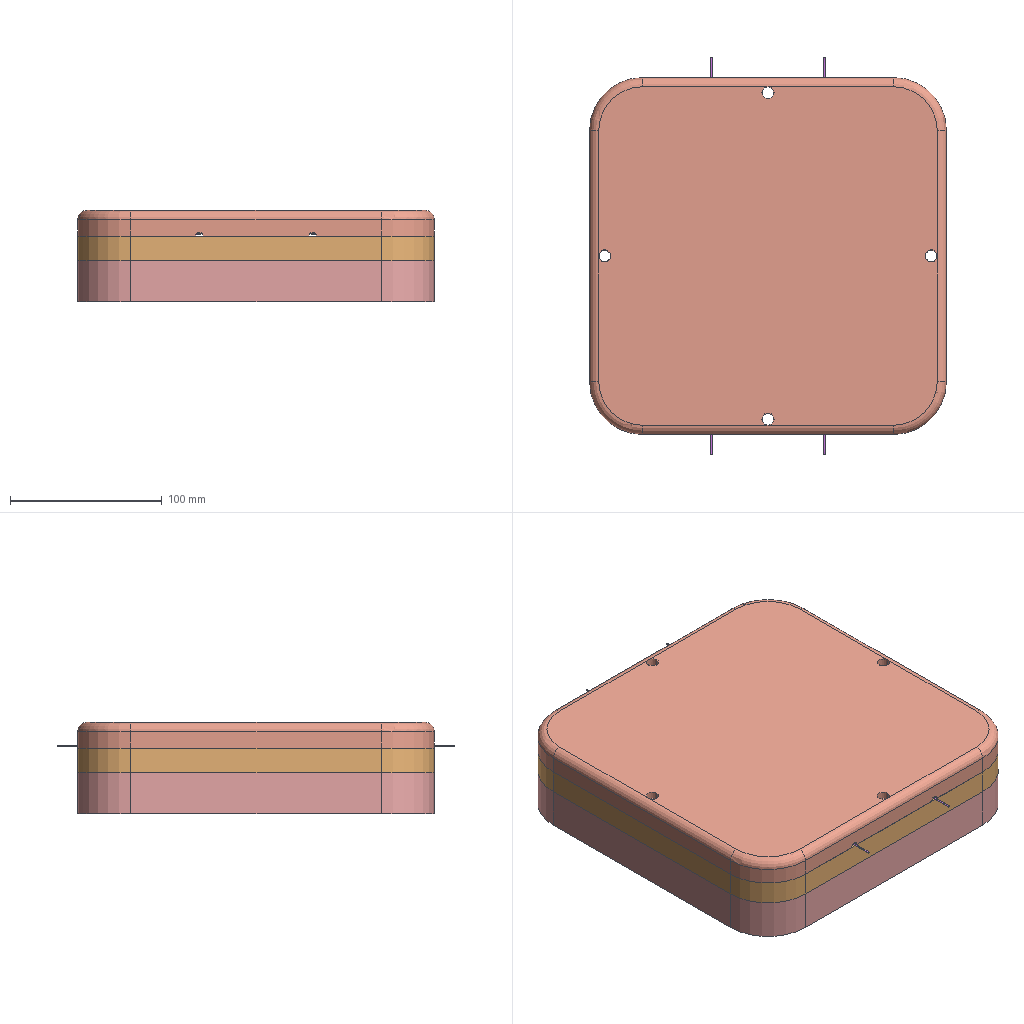Assembly | SolidWorks | 15 different items | 131 placed | box 235 x 262 x 60 mm
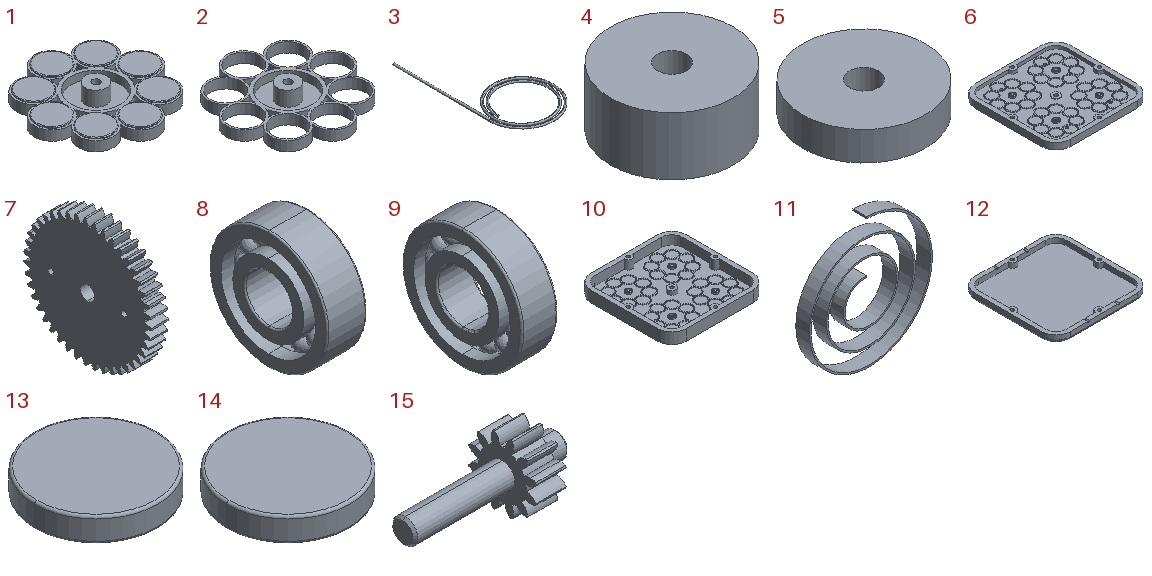Parts list (item | name | quantity | parent item | size | volume | features):
1 | (subassembly) | x4 | - | 100 x 100 x 14 mm | 35245 mm3 | features ReferencePattern 6, LocalCirPattern 1
2 | - | x4 | in 1 | 100 x 100 x 14 mm | 15045 mm3 | features ICE 2, Extrusion 1
3 | - | x4 | - | 33.004 x 66.506 x 1 mm | 182.398 mm3 | features Helix 1, ICE 1, Sweep 1
4 | - | x32 | - | 25.4 x 25.4 x 12 mm | 5741 mm3 | features Extrusion 1
5 | - | x32 | - | 25.4 x 25.4 x 6 mm | 2871 mm3 | features Extrusion 1
6 | - | x1 | - | 235 x 235 x 17 mm | 295331 mm3 | features ICE 7, Extrusion 1
7 | - | x4 | - | 6 x 44.961 x 44.988 mm | 8422 mm3 | features Boss 3, Cut 3, CirPattern 2, Fillet 2, ICE 1, Revolution 1
8 | - | x4 | - | 5 x 15 x 15 mm | 543.605 mm3 | features Revolution 3, CirPattern 1, Fillet 1
9 | - | x4 | - | 12 x 40 x 40 mm | 9102 mm3 | features Revolution 3, CirPattern 1, Fillet 1
10 | - | x1 | - | 235 x 235 x 27 mm | 476715 mm3 | features ICE 4, Extrusion 1
11 | - | x4 | - | 36.034 x 4 x 38.516 mm | 481.288 mm3 | features Helix 1, Sweep 1
12 | - | x1 | - | 235 x 235 x 17 mm | 369692 mm3 | features ICE 2, Extrusion 1, Fillet 1
13 | - | x16 | in 1 | 25.4 x 25.4 x 5 mm | 2525 mm3 | features Extrusion 1, Fillet 1
14 | - | x16 | in 1 | 25.4 x 25.4 x 5 mm | 2525 mm3 | features Extrusion 1, Fillet 1
15 | - | x4 | - | 31 x 13.609 x 13.609 mm | 1117 mm3 | features Boss 3, Cut 3, CirPattern 2, Fillet 2, ICE 2, Chamfer 1, Revolution 1
Mates (type | each side: item.copy, entity, surface, feature):
In the top assembly
Coincident | 10.1 face plane Boss-Extrude1 | 4.1 face plane Boss-Extrude1
Concentric | 10.1 face cylinder Boss-Extrude4 | 4.1 face cylinder Boss-Extrude1
Concentric | 10.1 face cylinder Boss-Extrude5 | 2.1 face cylinder Boss-Extrude1
DistanceDim | 4.2 face plane Boss-Extrude1 | 2.1 face plane Boss-Extrude1
Concentric | 10.1 face cylinder Boss-Extrude1 | 6.1 face cylinder Boss-Extrude1
Coincident | 10.1 face plane Boss-Extrude1 | 6.1 face plane Boss-Extrude1
Concentric | 6.1 face cylinder Boss-Extrude4 | 5.1 face cylinder Boss-Extrude1
Coincident | 6.1 face plane Boss-Extrude1 | 5.1 face plane Boss-Extrude1
Concentric | 6.1 face cylinder Cut-Extrude1 | 11.1 select_type:24
Coincident | 6.1 face plane Boss-Extrude1 | 11.1 face plane Sweep1
Coincident | 6.1 face plane Boss-Extrude1 | 11.2 face plane Sweep1
Concentric | 6.1 face cylinder Cut-Extrude1 | 11.2 select_type:24
Concentric | 6.1 face cylinder Cut-Extrude1 | 11.3 select_type:24
Coincident | 11.3 face plane Sweep1 | 11.2 face plane Sweep1
Concentric | 6.1 face cylinder Cut-Extrude1 | 11.4 select_type:24
Coincident | 11.1 face plane Sweep1 | 11.4 face plane Sweep1
Concentric | 6.1 face cylinder Boss-Extrude1 | 15.1 face cylinder Boss-Extrude2
Coincident | 15.1 face plane Base-Revolve | 7.1 face plane Base-Revolve
Coincident | 15.2 face plane Base-Revolve | 7.2 face plane Base-Revolve
Concentric | 6.1 face cylinder Cut-Extrude1 | 7.2 face cylinder Bore
Concentric | 6.1 face cylinder Cut-Extrude1 | 7.3 face cylinder Bore
Parallel | 15.3 face plane Base-Revolve | 7.3 face plane Base-Revolve
Coincident | 15.3 face plane Base-Revolve | 7.3 face plane Base-Revolve
Concentric | 6.1 face cylinder Cut-Extrude1 | 7.4 face cylinder Bore
Coincident | 15.4 face plane Base-Revolve | 7.4 face plane Base-Revolve
Concentric | 2.1 face cylinder Boss-Extrude1 | 9.1 face cylinder Revolve2
Coincident | 2.1 face plane Boss-Extrude3 | 9.1 face plane Revolve2
Concentric | 7.2 face cylinder Bore | 3.1 select_type:24
Parallel | 6.1 face plane Boss-Extrude1 | 3.1 select_type:24
Parallel | 6.1 face plane Boss-Extrude1 | 3.2 select_type:24
Tangent | 7.2 face plane Base-Revolve | 3.1 face surface:4006 Sweep1
Tangent | 7.4 face plane Base-Revolve | 3.3 face cylinder Boss-Extrude1
Concentric | 7.4 face cylinder Bore | 3.3 select_type:24
Parallel | 6.1 face plane Boss-Extrude1 | 3.3 select_type:24
Tangent | 7.3 face plane Base-Revolve | 3.4 face cylinder Boss-Extrude1
Concentric | 7.3 face cylinder Bore | 3.4 select_type:24
Parallel | 6.1 face plane Boss-Extrude1 | 3.4 select_type:24
Concentric | 7.1 face cylinder Bore | 3.2 select_type:24
Tangent | 7.1 face plane Base-Revolve | 3.2 face cylinder Boss-Extrude1
Concentric | 6.1 face cylinder Boss-Extrude6 | 8.1 face cylinder Revolve3
Coincident | 6.1 face plane Boss-Extrude1 | 8.1 face plane Revolve3
Coincident | 6.1 face plane Boss-Extrude1 | 12.1 face plane Boss-Extrude1 | 2 times
Coincident | 10.1 face plane Boss-Extrude2 | 6.1 face plane Boss-Extrude2
DistanceDim | 7.3 face plane Base-Revolve | 6.1 face plane Boss-Extrude6
Coincident | 6.1 face plane Boss-Extrude2 | 12.1 face plane Boss-Extrude2
Concentric | 6.1 face cylinder Cut-Extrude1 | 7.1 face cylinder Bore
In subassembly 1
Concentric | 2.2 face cylinder Boss-Extrude1 | 13.1 face cylinder Boss-Extrude1
Concentric | 2.2 face cylinder Boss-Extrude1 | 14.1 face cylinder Boss-Extrude1
Coincident | 14.1 face plane Boss-Extrude1 | 13.1 face plane Boss-Extrude1
DistanceDim | 13.1 face plane Boss-Extrude1 | 2.2 face plane Boss-Extrude1